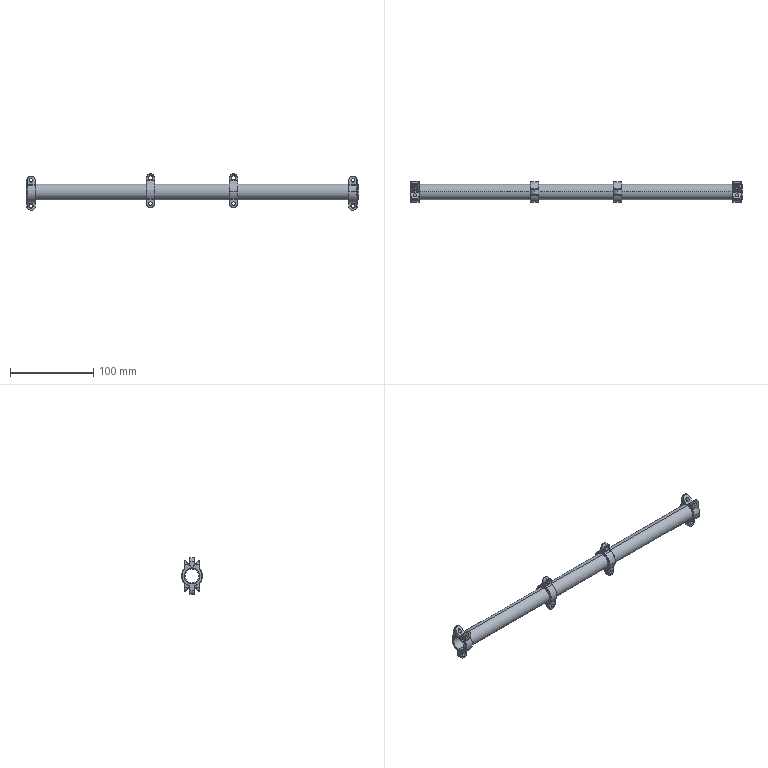Part | SolidWorks | features BaseBody 5 | 5 solids | 211 faces | box 400 x 25 x 44 mm | volume 39663 mm3 | cylinder 109 | spline 60 | plane 42 | commonest cylinder face diameters 1.016 x28 4 x16 4.166 x16 10 x16 25 x12 19.05 x11